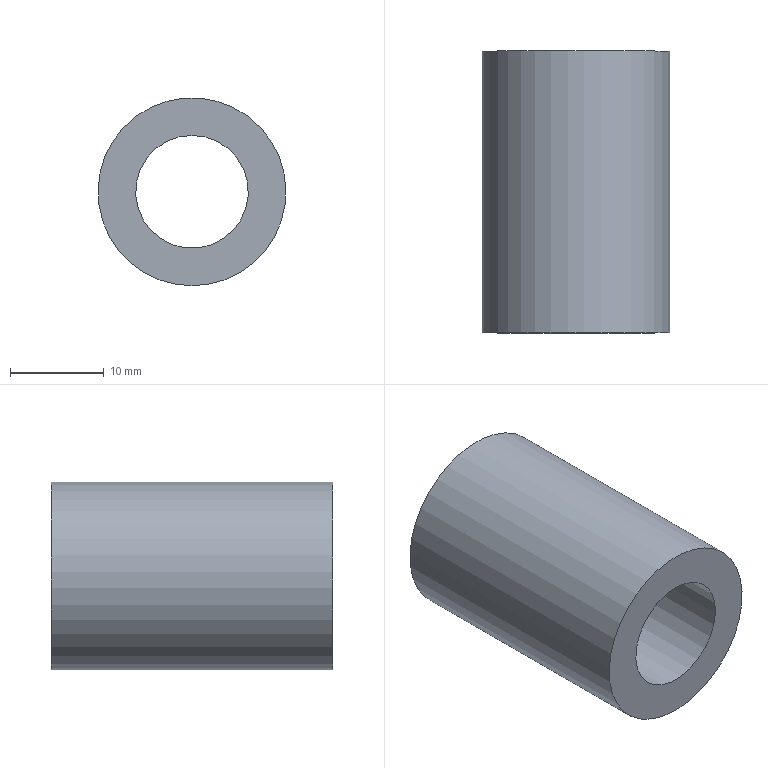Part | NX | features solid 2 | 1 solid | 4 faces | box 20 x 30 x 20 mm | volume 6032 mm3 | cylinder 2 | plane 2 | commonest cylinder face diameters 12 x1 20 x1
STEP:
#1=CARTESIAN_POINT('',(-160.,-130.,-40.));
#2=VERTEX_POINT('',#1);
#3=CARTESIAN_POINT('',(-160.,-130.,-30.));
#4=DIRECTION('',(0.,-1.,0.));
#5=DIRECTION('',(0.,0.,-1.));
#6=AXIS2_PLACEMENT_3D('',#3,#4,#5);
#7=CIRCLE('',#6,10.);
#8=EDGE_CURVE('',#2,#2,#7,.F.);
#9=ORIENTED_EDGE('',*,*,#8,.F.);
#10=EDGE_LOOP('',(#9));
#11=FACE_BOUND('',#10,.T.);
#12=CARTESIAN_POINT('',(-160.,-160.,-40.));
#13=VERTEX_POINT('',#12);
#14=CARTESIAN_POINT('',(-160.,-160.,-30.));
#15=DIRECTION('',(0.,-1.,0.));
#16=DIRECTION('',(0.,0.,-1.));
#17=AXIS2_PLACEMENT_3D('',#14,#15,#16);
#18=CIRCLE('',#17,10.);
#19=EDGE_CURVE('',#13,#13,#18,.F.);
#20=ORIENTED_EDGE('',*,*,#19,.T.);
#21=EDGE_LOOP('',(#20));
#22=FACE_BOUND('',#21,.T.);
#23=CARTESIAN_POINT('',(-160.,-160.,-30.));
#24=DIRECTION('',(0.,1.,0.));
#25=DIRECTION('',(0.,0.,1.));
#26=AXIS2_PLACEMENT_3D('',#23,#24,#25);
#27=CYLINDRICAL_SURFACE('',#26,10.);
#28=ADVANCED_FACE('',(#11,#22),#27,.T.);
#29=ORIENTED_EDGE('',*,*,#19,.F.);
#30=EDGE_LOOP('',(#29));
#31=FACE_BOUND('',#30,.T.);
#32=CARTESIAN_POINT('',(-160.,-160.,-24.));
#33=VERTEX_POINT('',#32);
#34=CARTESIAN_POINT('',(-160.,-160.,-30.));
#35=DIRECTION('',(0.,1.,0.));
#36=DIRECTION('',(0.,0.,1.));
#37=AXIS2_PLACEMENT_3D('',#34,#35,#36);
#38=CIRCLE('',#37,6.);
#39=EDGE_CURVE('',#33,#33,#38,.T.);
#40=ORIENTED_EDGE('',*,*,#39,.T.);
#41=EDGE_LOOP('',(#40));
#42=FACE_BOUND('',#41,.T.);
#43=CARTESIAN_POINT('',(-160.,-160.,-30.));
#44=DIRECTION('',(0.,-1.,0.));
#45=DIRECTION('',(0.,0.,-1.));
#46=AXIS2_PLACEMENT_3D('',#43,#44,#45);
#47=PLANE('',#46);
#48=ADVANCED_FACE('',(#31,#42),#47,.T.);
#49=ORIENTED_EDGE('',*,*,#8,.T.);
#50=EDGE_LOOP('',(#49));
#51=FACE_BOUND('',#50,.T.);
#52=CARTESIAN_POINT('',(-160.,-130.,-24.));
#53=VERTEX_POINT('',#52);
#54=CARTESIAN_POINT('',(-160.,-130.,-30.));
#55=DIRECTION('',(0.,1.,0.));
#56=DIRECTION('',(0.,0.,1.));
#57=AXIS2_PLACEMENT_3D('',#54,#55,#56);
#58=CIRCLE('',#57,6.);
#59=EDGE_CURVE('',#53,#53,#58,.T.);
#60=ORIENTED_EDGE('',*,*,#59,.F.);
#61=EDGE_LOOP('',(#60));
#62=FACE_BOUND('',#61,.T.);
#63=CARTESIAN_POINT('',(-160.,-130.,-30.));
#64=DIRECTION('',(0.,-1.,0.));
#65=DIRECTION('',(0.,0.,-1.));
#66=AXIS2_PLACEMENT_3D('',#63,#64,#65);
#67=PLANE('',#66);
#68=ADVANCED_FACE('',(#51,#62),#67,.F.);
#69=ORIENTED_EDGE('',*,*,#59,.T.);
#70=EDGE_LOOP('',(#69));
#71=FACE_BOUND('',#70,.T.);
#72=ORIENTED_EDGE('',*,*,#39,.F.);
#73=EDGE_LOOP('',(#72));
#74=FACE_BOUND('',#73,.T.);
#75=CARTESIAN_POINT('',(-160.,-160.,-30.));
#76=DIRECTION('',(0.,1.,0.));
#77=DIRECTION('',(0.,0.,1.));
#78=AXIS2_PLACEMENT_3D('',#75,#76,#77);
#79=CYLINDRICAL_SURFACE('',#78,6.);
#80=ADVANCED_FACE('',(#71,#74),#79,.F.);
#81=CLOSED_SHELL('',(#28,#48,#68,#80));
#82=MANIFOLD_SOLID_BREP('',#81);
#83=(LENGTH_UNIT()NAMED_UNIT(*)SI_UNIT(.MILLI.,.METRE.));
#84=UNCERTAINTY_MEASURE_WITH_UNIT(LENGTH_MEASURE(0.00001),#83,'','');
#85=(NAMED_UNIT(*)PLANE_ANGLE_UNIT()SI_UNIT($,.RADIAN.));
#86=(NAMED_UNIT(*)SI_UNIT($,.STERADIAN.)SOLID_ANGLE_UNIT());
#87=(GEOMETRIC_REPRESENTATION_CONTEXT(3)GLOBAL_UNCERTAINTY_ASSIGNED_CONTEXT((#84))GLOBAL_UNIT_ASSIGNED_CONTEXT((#83,#85,#86))REPRESENTATION_CONTEXT('',''));
#88=ADVANCED_BREP_SHAPE_REPRESENTATION('',(#82),#87);